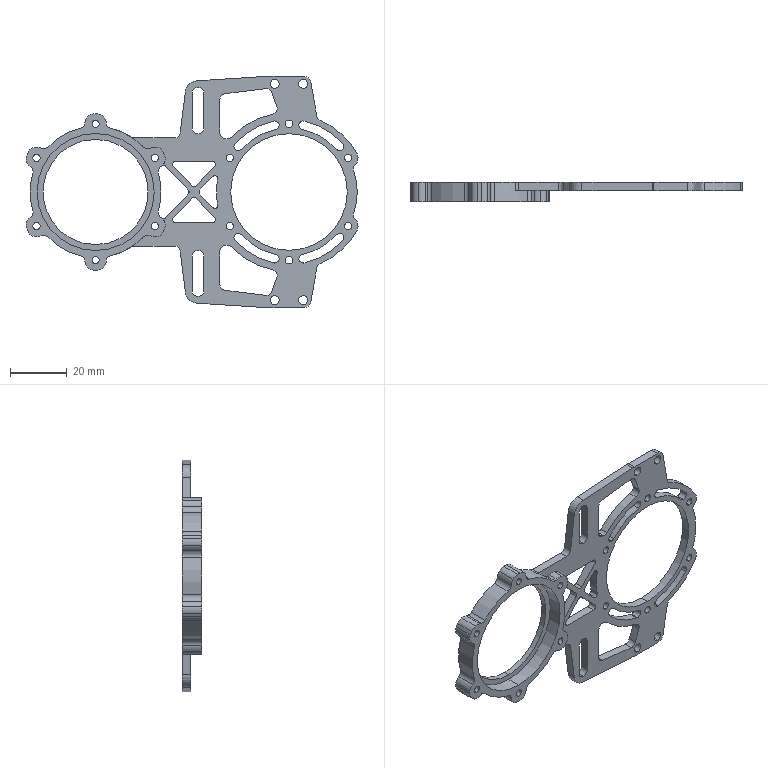Part | SolidWorks | features Fillet 6, ICE 4, Extrusion 1, MirrorPattern 1, PLine 1, Shell 1 | 1 solid | 201 faces | box 116.779 x 6.9 x 81.5 mm | volume 10389 mm3 | cylinder 165 | plane 36 | commonest cylinder face diameters 4 x31 2 x17 7.5 x14 2.5 x12 2.6 x12 3 x12